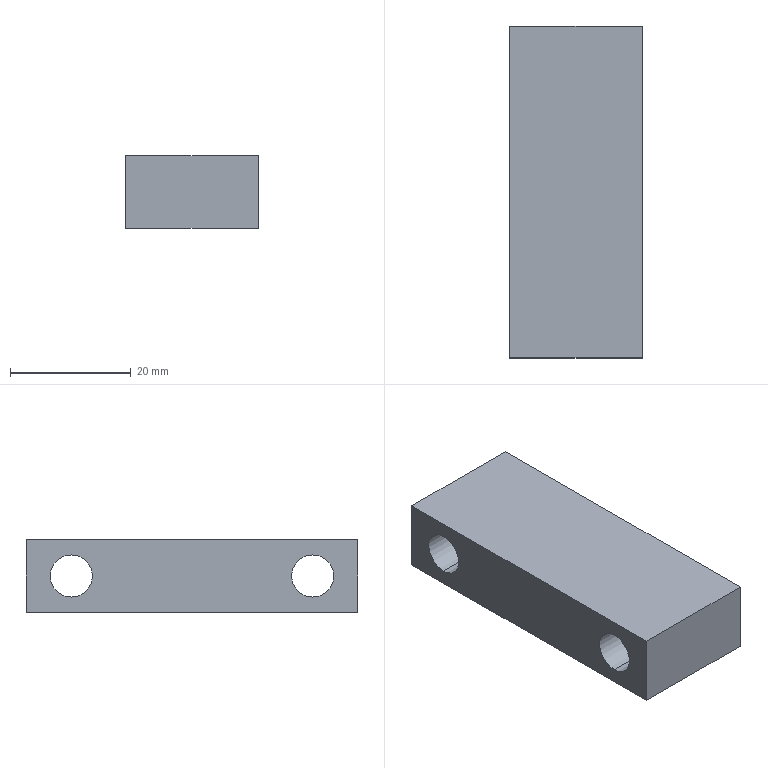Part | STEP file | CA-10-021Light Curtain Support Plate_Default | 1 solid | 10 faces | box 22 x 55 x 12 mm | volume 12827 mm3 | plane 6 | cylinder 4 | commonest cylinder face diameters 7 x4
STEP:
#1=CARTESIAN_POINT('',(0.,0.,0.));
#2=DIRECTION('',(0.,0.,1.));
#3=DIRECTION('',(1.,0.,0.));
#4=AXIS2_PLACEMENT_3D('',#1,#2,#3);
#5=CARTESIAN_POINT('',(11.,20.,9.5));
#6=VERTEX_POINT('',#5);
#7=CARTESIAN_POINT('',(-11.,20.,9.5));
#8=VERTEX_POINT('',#7);
#9=CARTESIAN_POINT('',(-11.,20.,9.5));
#10=DIRECTION('',(-1.,0.,0.));
#11=VECTOR('',#10,1.);
#12=LINE('',#9,#11);
#13=CARTESIAN_POINT('',(-11.,20.,6.));
#14=DIRECTION('',(-1.,0.,0.));
#15=DIRECTION('',(0.,0.,1.));
#16=AXIS2_PLACEMENT_3D('',#13,#14,#15);
#17=CYLINDRICAL_SURFACE('',#16,3.5);
#18=CARTESIAN_POINT('',(6.283,0.));
#19=DIRECTION('',(0.,1.));
#20=VECTOR('',#19,1.);
#21=LINE('',#18,#20);
#22=(GEOMETRIC_REPRESENTATION_CONTEXT(2)PARAMETRIC_REPRESENTATION_CONTEXT()REPRESENTATION_CONTEXT('',''));
#23=DEFINITIONAL_REPRESENTATION('',(#21),#22);
#24=PCURVE('',#17,#23);
#25=CARTESIAN_POINT('',(-11.,20.,6.));
#26=DIRECTION('',(-1.,0.,0.));
#27=DIRECTION('',(0.,0.,1.));
#28=AXIS2_PLACEMENT_3D('',#25,#26,#27);
#29=CYLINDRICAL_SURFACE('',#28,3.5);
#30=CARTESIAN_POINT('',(0.,0.));
#31=DIRECTION('',(0.,1.));
#32=VECTOR('',#31,1.);
#33=LINE('',#30,#32);
#34=(GEOMETRIC_REPRESENTATION_CONTEXT(2)PARAMETRIC_REPRESENTATION_CONTEXT()REPRESENTATION_CONTEXT('',''));
#35=DEFINITIONAL_REPRESENTATION('',(#33),#34);
#36=PCURVE('',#29,#35);
#37=SURFACE_CURVE('',#12,(#24,#36),.PCURVE_S1.);
#38=EDGE_CURVE('',#6,#8,#37,.T.);
#39=ORIENTED_EDGE('',*,*,#38,.T.);
#40=CARTESIAN_POINT('',(-11.,20.,2.5));
#41=VERTEX_POINT('',#40);
#42=CARTESIAN_POINT('',(-11.,20.,6.));
#43=DIRECTION('',(-1.,0.,0.));
#44=DIRECTION('',(0.,0.,1.));
#45=AXIS2_PLACEMENT_3D('',#42,#43,#44);
#46=CIRCLE('',#45,3.5);
#47=CARTESIAN_POINT('',(0.,0.));
#48=DIRECTION('',(1.,0.));
#49=VECTOR('',#48,1.);
#50=LINE('',#47,#49);
#51=(GEOMETRIC_REPRESENTATION_CONTEXT(2)PARAMETRIC_REPRESENTATION_CONTEXT()REPRESENTATION_CONTEXT('',''));
#52=DEFINITIONAL_REPRESENTATION('',(#50),#51);
#53=PCURVE('',#17,#52);
#54=CARTESIAN_POINT('',(-11.,27.5,12.));
#55=DIRECTION('',(1.,0.,0.));
#56=DIRECTION('',(0.,1.,0.));
#57=AXIS2_PLACEMENT_3D('',#54,#55,#56);
#58=PLANE('',#57);
#59=CARTESIAN_POINT('',(-7.5,-2.5));
#60=CARTESIAN_POINT('',(-1.438,-2.5));
#61=CARTESIAN_POINT('',(-4.469,-7.75));
#62=CARTESIAN_POINT('',(-7.5,-13.));
#63=CARTESIAN_POINT('',(-10.531,-7.75));
#64=CARTESIAN_POINT('',(-13.562,-2.5));
#65=CARTESIAN_POINT('',(-7.5,-2.5));
#66=(BOUNDED_CURVE()B_SPLINE_CURVE(2,(#59,#60,#61,#62,#63,#64,#65),.UNSPECIFIED.,.T.,.F.)B_SPLINE_CURVE_WITH_KNOTS((1,2,2,2,2,1),(-2.094,0.,2.094,4.189,6.283,8.378),.UNSPECIFIED.)CURVE()GEOMETRIC_REPRESENTATION_ITEM()RATIONAL_B_SPLINE_CURVE((1.,0.5,1.,0.5,1.,0.5,1.))REPRESENTATION_ITEM(''));
#67=(GEOMETRIC_REPRESENTATION_CONTEXT(2)PARAMETRIC_REPRESENTATION_CONTEXT()REPRESENTATION_CONTEXT('',''));
#68=DEFINITIONAL_REPRESENTATION('',(#66),#67);
#69=PCURVE('',#58,#68);
#70=SURFACE_CURVE('',#46,(#53,#69),.PCURVE_S1.);
#71=EDGE_CURVE('',#41,#8,#70,.T.);
#72=ORIENTED_EDGE('',*,*,#71,.F.);
#73=CARTESIAN_POINT('',(11.,20.,2.5));
#74=VERTEX_POINT('',#73);
#75=CARTESIAN_POINT('',(-11.,20.,2.5));
#76=DIRECTION('',(-1.,0.,0.));
#77=VECTOR('',#76,1.);
#78=LINE('',#75,#77);
#79=CARTESIAN_POINT('',(3.142,0.));
#80=DIRECTION('',(0.,1.));
#81=VECTOR('',#80,1.);
#82=LINE('',#79,#81);
#83=(GEOMETRIC_REPRESENTATION_CONTEXT(2)PARAMETRIC_REPRESENTATION_CONTEXT()REPRESENTATION_CONTEXT('',''));
#84=DEFINITIONAL_REPRESENTATION('',(#82),#83);
#85=PCURVE('',#17,#84);
#86=CARTESIAN_POINT('',(3.142,0.));
#87=DIRECTION('',(0.,1.));
#88=VECTOR('',#87,1.);
#89=LINE('',#86,#88);
#90=(GEOMETRIC_REPRESENTATION_CONTEXT(2)PARAMETRIC_REPRESENTATION_CONTEXT()REPRESENTATION_CONTEXT('',''));
#91=DEFINITIONAL_REPRESENTATION('',(#89),#90);
#92=PCURVE('',#29,#91);
#93=SURFACE_CURVE('',#78,(#85,#92),.PCURVE_S1.);
#94=EDGE_CURVE('',#74,#41,#93,.T.);
#95=ORIENTED_EDGE('',*,*,#94,.F.);
#96=CARTESIAN_POINT('',(11.,20.,6.));
#97=DIRECTION('',(-1.,0.,0.));
#98=DIRECTION('',(0.,0.,1.));
#99=AXIS2_PLACEMENT_3D('',#96,#97,#98);
#100=CIRCLE('',#99,3.5);
#101=CARTESIAN_POINT('',(0.,-22.));
#102=DIRECTION('',(1.,0.));
#103=VECTOR('',#102,1.);
#104=LINE('',#101,#103);
#105=(GEOMETRIC_REPRESENTATION_CONTEXT(2)PARAMETRIC_REPRESENTATION_CONTEXT()REPRESENTATION_CONTEXT('',''));
#106=DEFINITIONAL_REPRESENTATION('',(#104),#105);
#107=PCURVE('',#17,#106);
#108=CARTESIAN_POINT('',(11.,27.5,12.));
#109=DIRECTION('',(-1.,0.,0.));
#110=DIRECTION('',(0.,-1.,0.));
#111=AXIS2_PLACEMENT_3D('',#108,#109,#110);
#112=PLANE('',#111);
#113=CARTESIAN_POINT('',(7.5,-6.));
#114=DIRECTION('',(0.,1.));
#115=AXIS2_PLACEMENT_2D('',#113,#114);
#116=CIRCLE('',#115,3.5);
#117=(GEOMETRIC_REPRESENTATION_CONTEXT(2)PARAMETRIC_REPRESENTATION_CONTEXT()REPRESENTATION_CONTEXT('',''));
#118=DEFINITIONAL_REPRESENTATION('',(#116),#117);
#119=PCURVE('',#112,#118);
#120=SURFACE_CURVE('',#100,(#107,#119),.PCURVE_S1.);
#121=EDGE_CURVE('',#74,#6,#120,.T.);
#122=ORIENTED_EDGE('',*,*,#121,.T.);
#123=EDGE_LOOP('',(#39,#72,#95,#122));
#124=FACE_BOUND('',#123,.F.);
#125=ADVANCED_FACE('',(#124),#17,.F.);
#126=CARTESIAN_POINT('',(11.,-20.,9.5));
#127=VERTEX_POINT('',#126);
#128=CARTESIAN_POINT('',(-11.,-20.,9.5));
#129=VERTEX_POINT('',#128);
#130=CARTESIAN_POINT('',(-11.,-20.,9.5));
#131=DIRECTION('',(-1.,0.,0.));
#132=VECTOR('',#131,1.);
#133=LINE('',#130,#132);
#134=CARTESIAN_POINT('',(-11.,-20.,6.));
#135=DIRECTION('',(-1.,0.,0.));
#136=DIRECTION('',(0.,0.,1.));
#137=AXIS2_PLACEMENT_3D('',#134,#135,#136);
#138=CYLINDRICAL_SURFACE('',#137,3.5);
#139=CARTESIAN_POINT('',(6.283,0.));
#140=DIRECTION('',(0.,1.));
#141=VECTOR('',#140,1.);
#142=LINE('',#139,#141);
#143=(GEOMETRIC_REPRESENTATION_CONTEXT(2)PARAMETRIC_REPRESENTATION_CONTEXT()REPRESENTATION_CONTEXT('',''));
#144=DEFINITIONAL_REPRESENTATION('',(#142),#143);
#145=PCURVE('',#138,#144);
#146=CARTESIAN_POINT('',(-11.,-20.,6.));
#147=DIRECTION('',(-1.,0.,0.));
#148=DIRECTION('',(0.,0.,1.));
#149=AXIS2_PLACEMENT_3D('',#146,#147,#148);
#150=CYLINDRICAL_SURFACE('',#149,3.5);
#151=CARTESIAN_POINT('',(0.,0.));
#152=DIRECTION('',(0.,1.));
#153=VECTOR('',#152,1.);
#154=LINE('',#151,#153);
#155=(GEOMETRIC_REPRESENTATION_CONTEXT(2)PARAMETRIC_REPRESENTATION_CONTEXT()REPRESENTATION_CONTEXT('',''));
#156=DEFINITIONAL_REPRESENTATION('',(#154),#155);
#157=PCURVE('',#150,#156);
#158=SURFACE_CURVE('',#133,(#145,#157),.PCURVE_S1.);
#159=EDGE_CURVE('',#127,#129,#158,.T.);
#160=ORIENTED_EDGE('',*,*,#159,.T.);
#161=CARTESIAN_POINT('',(-11.,-20.,2.5));
#162=VERTEX_POINT('',#161);
#163=CARTESIAN_POINT('',(-11.,-20.,6.));
#164=DIRECTION('',(-1.,0.,0.));
#165=DIRECTION('',(0.,0.,1.));
#166=AXIS2_PLACEMENT_3D('',#163,#164,#165);
#167=CIRCLE('',#166,3.5);
#168=CARTESIAN_POINT('',(0.,0.));
#169=DIRECTION('',(1.,0.));
#170=VECTOR('',#169,1.);
#171=LINE('',#168,#170);
#172=(GEOMETRIC_REPRESENTATION_CONTEXT(2)PARAMETRIC_REPRESENTATION_CONTEXT()REPRESENTATION_CONTEXT('',''));
#173=DEFINITIONAL_REPRESENTATION('',(#171),#172);
#174=PCURVE('',#138,#173);
#175=CARTESIAN_POINT('',(-47.5,-2.5));
#176=CARTESIAN_POINT('',(-41.438,-2.5));
#177=CARTESIAN_POINT('',(-44.469,-7.75));
#178=CARTESIAN_POINT('',(-47.5,-13.));
#179=CARTESIAN_POINT('',(-50.531,-7.75));
#180=CARTESIAN_POINT('',(-53.562,-2.5));
#181=CARTESIAN_POINT('',(-47.5,-2.5));
#182=(BOUNDED_CURVE()B_SPLINE_CURVE(2,(#175,#176,#177,#178,#179,#180,#181),.UNSPECIFIED.,.T.,.F.)B_SPLINE_CURVE_WITH_KNOTS((1,2,2,2,2,1),(-2.094,0.,2.094,4.189,6.283,8.378),.UNSPECIFIED.)CURVE()GEOMETRIC_REPRESENTATION_ITEM()RATIONAL_B_SPLINE_CURVE((1.,0.5,1.,0.5,1.,0.5,1.))REPRESENTATION_ITEM(''));
#183=(GEOMETRIC_REPRESENTATION_CONTEXT(2)PARAMETRIC_REPRESENTATION_CONTEXT()REPRESENTATION_CONTEXT('',''));
#184=DEFINITIONAL_REPRESENTATION('',(#182),#183);
#185=PCURVE('',#58,#184);
#186=SURFACE_CURVE('',#167,(#174,#185),.PCURVE_S1.);
#187=EDGE_CURVE('',#162,#129,#186,.T.);
#188=ORIENTED_EDGE('',*,*,#187,.F.);
#189=CARTESIAN_POINT('',(11.,-20.,2.5));
#190=VERTEX_POINT('',#189);
#191=CARTESIAN_POINT('',(-11.,-20.,2.5));
#192=DIRECTION('',(-1.,0.,0.));
#193=VECTOR('',#192,1.);
#194=LINE('',#191,#193);
#195=CARTESIAN_POINT('',(3.142,0.));
#196=DIRECTION('',(0.,1.));
#197=VECTOR('',#196,1.);
#198=LINE('',#195,#197);
#199=(GEOMETRIC_REPRESENTATION_CONTEXT(2)PARAMETRIC_REPRESENTATION_CONTEXT()REPRESENTATION_CONTEXT('',''));
#200=DEFINITIONAL_REPRESENTATION('',(#198),#199);
#201=PCURVE('',#138,#200);
#202=CARTESIAN_POINT('',(3.142,0.));
#203=DIRECTION('',(0.,1.));
#204=VECTOR('',#203,1.);
#205=LINE('',#202,#204);
#206=(GEOMETRIC_REPRESENTATION_CONTEXT(2)PARAMETRIC_REPRESENTATION_CONTEXT()REPRESENTATION_CONTEXT('',''));
#207=DEFINITIONAL_REPRESENTATION('',(#205),#206);
#208=PCURVE('',#150,#207);
#209=SURFACE_CURVE('',#194,(#201,#208),.PCURVE_S1.);
#210=EDGE_CURVE('',#190,#162,#209,.T.);
#211=ORIENTED_EDGE('',*,*,#210,.F.);
#212=CARTESIAN_POINT('',(11.,-20.,6.));
#213=DIRECTION('',(-1.,0.,0.));
#214=DIRECTION('',(0.,0.,1.));
#215=AXIS2_PLACEMENT_3D('',#212,#213,#214);
#216=CIRCLE('',#215,3.5);
#217=CARTESIAN_POINT('',(0.,-22.));
#218=DIRECTION('',(1.,0.));
#219=VECTOR('',#218,1.);
#220=LINE('',#217,#219);
#221=(GEOMETRIC_REPRESENTATION_CONTEXT(2)PARAMETRIC_REPRESENTATION_CONTEXT()REPRESENTATION_CONTEXT('',''));
#222=DEFINITIONAL_REPRESENTATION('',(#220),#221);
#223=PCURVE('',#138,#222);
#224=CARTESIAN_POINT('',(47.5,-6.));
#225=DIRECTION('',(0.,1.));
#226=AXIS2_PLACEMENT_2D('',#224,#225);
#227=CIRCLE('',#226,3.5);
#228=(GEOMETRIC_REPRESENTATION_CONTEXT(2)PARAMETRIC_REPRESENTATION_CONTEXT()REPRESENTATION_CONTEXT('',''));
#229=DEFINITIONAL_REPRESENTATION('',(#227),#228);
#230=PCURVE('',#112,#229);
#231=SURFACE_CURVE('',#216,(#223,#230),.PCURVE_S1.);
#232=EDGE_CURVE('',#190,#127,#231,.T.);
#233=ORIENTED_EDGE('',*,*,#232,.T.);
#234=EDGE_LOOP('',(#160,#188,#211,#233));
#235=FACE_BOUND('',#234,.F.);
#236=ADVANCED_FACE('',(#235),#138,.F.);
#237=CARTESIAN_POINT('',(11.,20.,6.));
#238=DIRECTION('',(-1.,0.,0.));
#239=DIRECTION('',(0.,0.,1.));
#240=AXIS2_PLACEMENT_3D('',#237,#238,#239);
#241=CIRCLE('',#240,3.5);
#242=CARTESIAN_POINT('',(7.5,-6.));
#243=DIRECTION('',(0.,1.));
#244=AXIS2_PLACEMENT_2D('',#242,#243);
#245=CIRCLE('',#244,3.5);
#246=(GEOMETRIC_REPRESENTATION_CONTEXT(2)PARAMETRIC_REPRESENTATION_CONTEXT()REPRESENTATION_CONTEXT('',''));
#247=DEFINITIONAL_REPRESENTATION('',(#245),#246);
#248=PCURVE('',#112,#247);
#249=CARTESIAN_POINT('',(0.,-22.));
#250=DIRECTION('',(1.,0.));
#251=VECTOR('',#250,1.);
#252=LINE('',#249,#251);
#253=(GEOMETRIC_REPRESENTATION_CONTEXT(2)PARAMETRIC_REPRESENTATION_CONTEXT()REPRESENTATION_CONTEXT('',''));
#254=DEFINITIONAL_REPRESENTATION('',(#252),#253);
#255=PCURVE('',#29,#254);
#256=SURFACE_CURVE('',#241,(#248,#255),.PCURVE_S1.);
#257=EDGE_CURVE('',#6,#74,#256,.T.);
#258=ORIENTED_EDGE('',*,*,#257,.T.);
#259=ORIENTED_EDGE('',*,*,#121,.T.);
#260=EDGE_LOOP('',(#258,#259));
#261=FACE_BOUND('',#260,.T.);
#262=CARTESIAN_POINT('',(11.,-20.,6.));
#263=DIRECTION('',(-1.,0.,0.));
#264=DIRECTION('',(0.,0.,1.));
#265=AXIS2_PLACEMENT_3D('',#262,#263,#264);
#266=CIRCLE('',#265,3.5);
#267=CARTESIAN_POINT('',(47.5,-6.));
#268=DIRECTION('',(0.,1.));
#269=AXIS2_PLACEMENT_2D('',#267,#268);
#270=CIRCLE('',#269,3.5);
#271=(GEOMETRIC_REPRESENTATION_CONTEXT(2)PARAMETRIC_REPRESENTATION_CONTEXT()REPRESENTATION_CONTEXT('',''));
#272=DEFINITIONAL_REPRESENTATION('',(#270),#271);
#273=PCURVE('',#112,#272);
#274=CARTESIAN_POINT('',(0.,-22.));
#275=DIRECTION('',(1.,0.));
#276=VECTOR('',#275,1.);
#277=LINE('',#274,#276);
#278=(GEOMETRIC_REPRESENTATION_CONTEXT(2)PARAMETRIC_REPRESENTATION_CONTEXT()REPRESENTATION_CONTEXT('',''));
#279=DEFINITIONAL_REPRESENTATION('',(#277),#278);
#280=PCURVE('',#150,#279);
#281=SURFACE_CURVE('',#266,(#273,#280),.PCURVE_S1.);
#282=EDGE_CURVE('',#127,#190,#281,.T.);
#283=ORIENTED_EDGE('',*,*,#282,.T.);
#284=ORIENTED_EDGE('',*,*,#232,.T.);
#285=EDGE_LOOP('',(#283,#284));
#286=FACE_BOUND('',#285,.T.);
#287=CARTESIAN_POINT('',(11.,-27.5,0.));
#288=VERTEX_POINT('',#287);
#289=CARTESIAN_POINT('',(11.,27.5,0.));
#290=VERTEX_POINT('',#289);
#291=CARTESIAN_POINT('',(11.,27.5,0.));
#292=DIRECTION('',(0.,1.,0.));
#293=VECTOR('',#292,1.);
#294=LINE('',#291,#293);
#295=CARTESIAN_POINT('',(0.,-12.));
#296=DIRECTION('',(-1.,0.));
#297=VECTOR('',#296,1.);
#298=LINE('',#295,#297);
#299=(GEOMETRIC_REPRESENTATION_CONTEXT(2)PARAMETRIC_REPRESENTATION_CONTEXT()REPRESENTATION_CONTEXT('',''));
#300=DEFINITIONAL_REPRESENTATION('',(#298),#299);
#301=PCURVE('',#112,#300);
#302=CARTESIAN_POINT('',(0.,0.,0.));
#303=DIRECTION('',(0.,0.,1.));
#304=DIRECTION('',(1.,0.,0.));
#305=AXIS2_PLACEMENT_3D('',#302,#303,#304);
#306=PLANE('',#305);
#307=CARTESIAN_POINT('',(11.,27.5));
#308=DIRECTION('',(0.,1.));
#309=VECTOR('',#308,1.);
#310=LINE('',#307,#309);
#311=(GEOMETRIC_REPRESENTATION_CONTEXT(2)PARAMETRIC_REPRESENTATION_CONTEXT()REPRESENTATION_CONTEXT('',''));
#312=DEFINITIONAL_REPRESENTATION('',(#310),#311);
#313=PCURVE('',#306,#312);
#314=SURFACE_CURVE('',#294,(#301,#313),.PCURVE_S1.);
#315=EDGE_CURVE('',#288,#290,#314,.T.);
#316=ORIENTED_EDGE('',*,*,#315,.T.);
#317=CARTESIAN_POINT('',(11.,27.5,12.));
#318=VERTEX_POINT('',#317);
#319=CARTESIAN_POINT('',(11.,27.5,12.));
#320=DIRECTION('',(0.,0.,-1.));
#321=VECTOR('',#320,1.);
#322=LINE('',#319,#321);
#323=CARTESIAN_POINT('',(0.,0.));
#324=DIRECTION('',(0.,-1.));
#325=VECTOR('',#324,1.);
#326=LINE('',#323,#325);
#327=(GEOMETRIC_REPRESENTATION_CONTEXT(2)PARAMETRIC_REPRESENTATION_CONTEXT()REPRESENTATION_CONTEXT('',''));
#328=DEFINITIONAL_REPRESENTATION('',(#326),#327);
#329=PCURVE('',#112,#328);
#330=CARTESIAN_POINT('',(-11.,27.5,12.));
#331=DIRECTION('',(0.,-1.,0.));
#332=DIRECTION('',(0.,0.,-1.));
#333=AXIS2_PLACEMENT_3D('',#330,#331,#332);
#334=PLANE('',#333);
#335=CARTESIAN_POINT('',(0.,22.));
#336=DIRECTION('',(1.,0.));
#337=VECTOR('',#336,1.);
#338=LINE('',#335,#337);
#339=(GEOMETRIC_REPRESENTATION_CONTEXT(2)PARAMETRIC_REPRESENTATION_CONTEXT()REPRESENTATION_CONTEXT('',''));
#340=DEFINITIONAL_REPRESENTATION('',(#338),#339);
#341=PCURVE('',#334,#340);
#342=SURFACE_CURVE('',#322,(#329,#341),.PCURVE_S1.);
#343=EDGE_CURVE('',#318,#290,#342,.T.);
#344=ORIENTED_EDGE('',*,*,#343,.F.);
#345=CARTESIAN_POINT('',(11.,-27.5,12.));
#346=VERTEX_POINT('',#345);
#347=CARTESIAN_POINT('',(11.,27.5,12.));
#348=DIRECTION('',(0.,1.,0.));
#349=VECTOR('',#348,1.);
#350=LINE('',#347,#349);
#351=CARTESIAN_POINT('',(0.,0.));
#352=DIRECTION('',(-1.,0.));
#353=VECTOR('',#352,1.);
#354=LINE('',#351,#353);
#355=(GEOMETRIC_REPRESENTATION_CONTEXT(2)PARAMETRIC_REPRESENTATION_CONTEXT()REPRESENTATION_CONTEXT('',''));
#356=DEFINITIONAL_REPRESENTATION('',(#354),#355);
#357=PCURVE('',#112,#356);
#358=CARTESIAN_POINT('',(0.,0.,12.));
#359=DIRECTION('',(0.,0.,1.));
#360=DIRECTION('',(1.,0.,0.));
#361=AXIS2_PLACEMENT_3D('',#358,#359,#360);
#362=PLANE('',#361);
#363=CARTESIAN_POINT('',(11.,27.5));
#364=DIRECTION('',(0.,1.));
#365=VECTOR('',#364,1.);
#366=LINE('',#363,#365);
#367=(GEOMETRIC_REPRESENTATION_CONTEXT(2)PARAMETRIC_REPRESENTATION_CONTEXT()REPRESENTATION_CONTEXT('',''));
#368=DEFINITIONAL_REPRESENTATION('',(#366),#367);
#369=PCURVE('',#362,#368);
#370=SURFACE_CURVE('',#350,(#357,#369),.PCURVE_S1.);
#371=EDGE_CURVE('',#346,#318,#370,.T.);
#372=ORIENTED_EDGE('',*,*,#371,.F.);
#373=CARTESIAN_POINT('',(11.,-27.5,12.));
#374=DIRECTION('',(0.,0.,-1.));
#375=VECTOR('',#374,1.);
#376=LINE('',#373,#375);
#377=CARTESIAN_POINT('',(55.,0.));
#378=DIRECTION('',(0.,-1.));
#379=VECTOR('',#378,1.);
#380=LINE('',#377,#379);
#381=(GEOMETRIC_REPRESENTATION_CONTEXT(2)PARAMETRIC_REPRESENTATION_CONTEXT()REPRESENTATION_CONTEXT('',''));
#382=DEFINITIONAL_REPRESENTATION('',(#380),#381);
#383=PCURVE('',#112,#382);
#384=CARTESIAN_POINT('',(-11.,-27.5,12.));
#385=DIRECTION('',(0.,1.,0.));
#386=DIRECTION('',(0.,0.,1.));
#387=AXIS2_PLACEMENT_3D('',#384,#385,#386);
#388=PLANE('',#387);
#389=CARTESIAN_POINT('',(0.,22.));
#390=DIRECTION('',(-1.,0.));
#391=VECTOR('',#390,1.);
#392=LINE('',#389,#391);
#393=(GEOMETRIC_REPRESENTATION_CONTEXT(2)PARAMETRIC_REPRESENTATION_CONTEXT()REPRESENTATION_CONTEXT('',''));
#394=DEFINITIONAL_REPRESENTATION('',(#392),#393);
#395=PCURVE('',#388,#394);
#396=SURFACE_CURVE('',#376,(#383,#395),.PCURVE_S1.);
#397=EDGE_CURVE('',#346,#288,#396,.T.);
#398=ORIENTED_EDGE('',*,*,#397,.T.);
#399=EDGE_LOOP('',(#316,#344,#372,#398));
#400=FACE_BOUND('',#399,.T.);
#401=ADVANCED_FACE('',(#261,#286,#400),#112,.F.);
#402=CARTESIAN_POINT('',(-11.,27.5,0.));
#403=VERTEX_POINT('',#402);
#404=CARTESIAN_POINT('',(-11.,27.5,0.));
#405=DIRECTION('',(-1.,0.,0.));
#406=VECTOR('',#405,1.);
#407=LINE('',#404,#406);
#408=CARTESIAN_POINT('',(12.,0.));
#409=DIRECTION('',(0.,-1.));
#410=VECTOR('',#409,1.);
#411=LINE('',#408,#410);
#412=(GEOMETRIC_REPRESENTATION_CONTEXT(2)PARAMETRIC_REPRESENTATION_CONTEXT()REPRESENTATION_CONTEXT('',''));
#413=DEFINITIONAL_REPRESENTATION('',(#411),#412);
#414=PCURVE('',#334,#413);
#415=CARTESIAN_POINT('',(-11.,27.5));
#416=DIRECTION('',(-1.,0.));
#417=VECTOR('',#416,1.);
#418=LINE('',#415,#417);
#419=(GEOMETRIC_REPRESENTATION_CONTEXT(2)PARAMETRIC_REPRESENTATION_CONTEXT()REPRESENTATION_CONTEXT('',''));
#420=DEFINITIONAL_REPRESENTATION('',(#418),#419);
#421=PCURVE('',#306,#420);
#422=SURFACE_CURVE('',#407,(#414,#421),.PCURVE_S1.);
#423=EDGE_CURVE('',#290,#403,#422,.T.);
#424=ORIENTED_EDGE('',*,*,#423,.T.);
#425=CARTESIAN_POINT('',(-11.,27.5,12.));
#426=VERTEX_POINT('',#425);
#427=CARTESIAN_POINT('',(-11.,27.5,12.));
#428=DIRECTION('',(0.,0.,-1.));
#429=VECTOR('',#428,1.);
#430=LINE('',#427,#429);
#431=CARTESIAN_POINT('',(0.,0.));
#432=DIRECTION('',(1.,0.));
#433=VECTOR('',#432,1.);
#434=LINE('',#431,#433);
#435=(GEOMETRIC_REPRESENTATION_CONTEXT(2)PARAMETRIC_REPRESENTATION_CONTEXT()REPRESENTATION_CONTEXT('',''));
#436=DEFINITIONAL_REPRESENTATION('',(#434),#435);
#437=PCURVE('',#334,#436);
#438=CARTESIAN_POINT('',(0.,0.));
#439=DIRECTION('',(0.,-1.));
#440=VECTOR('',#439,1.);
#441=LINE('',#438,#440);
#442=(GEOMETRIC_REPRESENTATION_CONTEXT(2)PARAMETRIC_REPRESENTATION_CONTEXT()REPRESENTATION_CONTEXT('',''));
#443=DEFINITIONAL_REPRESENTATION('',(#441),#442);
#444=PCURVE('',#58,#443);
#445=SURFACE_CURVE('',#430,(#437,#444),.PCURVE_S1.);
#446=EDGE_CURVE('',#426,#403,#445,.T.);
#447=ORIENTED_EDGE('',*,*,#446,.F.);
#448=CARTESIAN_POINT('',(-11.,27.5,12.));
#449=DIRECTION('',(-1.,0.,0.));
#450=VECTOR('',#449,1.);
#451=LINE('',#448,#450);
#452=CARTESIAN_POINT('',(0.,0.));
#453=DIRECTION('',(0.,-1.));
#454=VECTOR('',#453,1.);
#455=LINE('',#452,#454);
#456=(GEOMETRIC_REPRESENTATION_CONTEXT(2)PARAMETRIC_REPRESENTATION_CONTEXT()REPRESENTATION_CONTEXT('',''));
#457=DEFINITIONAL_REPRESENTATION('',(#455),#456);
#458=PCURVE('',#334,#457);
#459=CARTESIAN_POINT('',(-11.,27.5));
#460=DIRECTION('',(-1.,0.));
#461=VECTOR('',#460,1.);
#462=LINE('',#459,#461);
#463=(GEOMETRIC_REPRESENTATION_CONTEXT(2)PARAMETRIC_REPRESENTATION_CONTEXT()REPRESENTATION_CONTEXT('',''));
#464=DEFINITIONAL_REPRESENTATION('',(#462),#463);
#465=PCURVE('',#362,#464);
#466=SURFACE_CURVE('',#451,(#458,#465),.PCURVE_S1.);
#467=EDGE_CURVE('',#318,#426,#466,.T.);
#468=ORIENTED_EDGE('',*,*,#467,.F.);
#469=ORIENTED_EDGE('',*,*,#343,.T.);
#470=EDGE_LOOP('',(#424,#447,#468,#469));
#471=FACE_BOUND('',#470,.T.);
#472=ADVANCED_FACE('',(#471),#334,.F.);
#473=CARTESIAN_POINT('',(-11.,20.,6.));
#474=DIRECTION('',(-1.,0.,0.));
#475=DIRECTION('',(0.,0.,1.));
#476=AXIS2_PLACEMENT_3D('',#473,#474,#475);
#477=CIRCLE('',#476,3.5);
#478=CARTESIAN_POINT('',(-7.5,-2.5));
#479=CARTESIAN_POINT('',(-1.438,-2.5));
#480=CARTESIAN_POINT('',(-4.469,-7.75));
#481=CARTESIAN_POINT('',(-7.5,-13.));
#482=CARTESIAN_POINT('',(-10.531,-7.75));
#483=CARTESIAN_POINT('',(-13.562,-2.5));
#484=CARTESIAN_POINT('',(-7.5,-2.5));
#485=(BOUNDED_CURVE()B_SPLINE_CURVE(2,(#478,#479,#480,#481,#482,#483,#484),.UNSPECIFIED.,.T.,.F.)B_SPLINE_CURVE_WITH_KNOTS((1,2,2,2,2,1),(-2.094,0.,2.094,4.189,6.283,8.378),.UNSPECIFIED.)CURVE()GEOMETRIC_REPRESENTATION_ITEM()RATIONAL_B_SPLINE_CURVE((1.,0.5,1.,0.5,1.,0.5,1.))REPRESENTATION_ITEM(''));
#486=(GEOMETRIC_REPRESENTATION_CONTEXT(2)PARAMETRIC_REPRESENTATION_CONTEXT()REPRESENTATION_CONTEXT('',''));
#487=DEFINITIONAL_REPRESENTATION('',(#485),#486);
#488=PCURVE('',#58,#487);
#489=CARTESIAN_POINT('',(0.,0.));
#490=DIRECTION('',(1.,0.));
#491=VECTOR('',#490,1.);
#492=LINE('',#489,#491);
#493=(GEOMETRIC_REPRESENTATION_CONTEXT(2)PARAMETRIC_REPRESENTATION_CONTEXT()REPRESENTATION_CONTEXT('',''));
#494=DEFINITIONAL_REPRESENTATION('',(#492),#493);
#495=PCURVE('',#29,#494);
#496=SURFACE_CURVE('',#477,(#488,#495),.PCURVE_S1.);
#497=EDGE_CURVE('',#8,#41,#496,.T.);
#498=ORIENTED_EDGE('',*,*,#497,.F.);
#499=ORIENTED_EDGE('',*,*,#71,.F.);
#500=EDGE_LOOP('',(#498,#499));
#501=FACE_BOUND('',#500,.T.);
#502=CARTESIAN_POINT('',(-11.,-20.,6.));
#503=DIRECTION('',(-1.,0.,0.));
#504=DIRECTION('',(0.,0.,1.));
#505=AXIS2_PLACEMENT_3D('',#502,#503,#504);
#506=CIRCLE('',#505,3.5);
#507=CARTESIAN_POINT('',(-47.5,-2.5));
#508=CARTESIAN_POINT('',(-41.438,-2.5));
#509=CARTESIAN_POINT('',(-44.469,-7.75));
#510=CARTESIAN_POINT('',(-47.5,-13.));
#511=CARTESIAN_POINT('',(-50.531,-7.75));
#512=CARTESIAN_POINT('',(-53.562,-2.5));
#513=CARTESIAN_POINT('',(-47.5,-2.5));
#514=(BOUNDED_CURVE()B_SPLINE_CURVE(2,(#507,#508,#509,#510,#511,#512,#513),.UNSPECIFIED.,.T.,.F.)B_SPLINE_CURVE_WITH_KNOTS((1,2,2,2,2,1),(-2.094,0.,2.094,4.189,6.283,8.378),.UNSPECIFIED.)CURVE()GEOMETRIC_REPRESENTATION_ITEM()RATIONAL_B_SPLINE_CURVE((1.,0.5,1.,0.5,1.,0.5,1.))REPRESENTATION_ITEM(''));
#515=(GEOMETRIC_REPRESENTATION_CONTEXT(2)PARAMETRIC_REPRESENTATION_CONTEXT()REPRESENTATION_CONTEXT('',''));
#516=DEFINITIONAL_REPRESENTATION('',(#514),#515);
#517=PCURVE('',#58,#516);
#518=CARTESIAN_POINT('',(0.,0.));
#519=DIRECTION('',(1.,0.));
#520=VECTOR('',#519,1.);
#521=LINE('',#518,#520);
#522=(GEOMETRIC_REPRESENTATION_CONTEXT(2)PARAMETRIC_REPRESENTATION_CONTEXT()REPRESENTATION_CONTEXT('',''));
#523=DEFINITIONAL_REPRESENTATION('',(#521),#522);
#524=PCURVE('',#150,#523);
#525=SURFACE_CURVE('',#506,(#517,#524),.PCURVE_S1.);
#526=EDGE_CURVE('',#129,#162,#525,.T.);
#527=ORIENTED_EDGE('',*,*,#526,.F.);
#528=ORIENTED_EDGE('',*,*,#187,.F.);
#529=EDGE_LOOP('',(#527,#528));
#530=FACE_BOUND('',#529,.T.);
#531=CARTESIAN_POINT('',(-11.,-27.5,0.));
#532=VERTEX_POINT('',#531);
#533=CARTESIAN_POINT('',(-11.,27.5,0.));
#534=DIRECTION('',(0.,-1.,0.));
#535=VECTOR('',#534,1.);
#536=LINE('',#533,#535);
#537=CARTESIAN_POINT('',(0.,-12.));
#538=DIRECTION('',(-1.,0.));
#539=VECTOR('',#538,1.);
#540=LINE('',#537,#539);
#541=(GEOMETRIC_REPRESENTATION_CONTEXT(2)PARAMETRIC_REPRESENTATION_CONTEXT()REPRESENTATION_CONTEXT('',''));
#542=DEFINITIONAL_REPRESENTATION('',(#540),#541);
#543=PCURVE('',#58,#542);
#544=CARTESIAN_POINT('',(-11.,27.5));
#545=DIRECTION('',(0.,-1.));
#546=VECTOR('',#545,1.);
#547=LINE('',#544,#546);
#548=(GEOMETRIC_REPRESENTATION_CONTEXT(2)PARAMETRIC_REPRESENTATION_CONTEXT()REPRESENTATION_CONTEXT('',''));
#549=DEFINITIONAL_REPRESENTATION('',(#547),#548);
#550=PCURVE('',#306,#549);
#551=SURFACE_CURVE('',#536,(#543,#550),.PCURVE_S1.);
#552=EDGE_CURVE('',#403,#532,#551,.T.);
#553=ORIENTED_EDGE('',*,*,#552,.T.);
#554=CARTESIAN_POINT('',(-11.,-27.5,12.));
#555=VERTEX_POINT('',#554);
#556=CARTESIAN_POINT('',(-11.,-27.5,12.));
#557=DIRECTION('',(0.,0.,-1.));
#558=VECTOR('',#557,1.);
#559=LINE('',#556,#558);
#560=CARTESIAN_POINT('',(-55.,0.));
#561=DIRECTION('',(0.,-1.));
#562=VECTOR('',#561,1.);
#563=LINE('',#560,#562);
#564=(GEOMETRIC_REPRESENTATION_CONTEXT(2)PARAMETRIC_REPRESENTATION_CONTEXT()REPRESENTATION_CONTEXT('',''));
#565=DEFINITIONAL_REPRESENTATION('',(#563),#564);
#566=PCURVE('',#58,#565);
#567=CARTESIAN_POINT('',(0.,0.));
#568=DIRECTION('',(-1.,0.));
#569=VECTOR('',#568,1.);
#570=LINE('',#567,#569);
#571=(GEOMETRIC_REPRESENTATION_CONTEXT(2)PARAMETRIC_REPRESENTATION_CONTEXT()REPRESENTATION_CONTEXT('',''));
#572=DEFINITIONAL_REPRESENTATION('',(#570),#571);
#573=PCURVE('',#388,#572);
#574=SURFACE_CURVE('',#559,(#566,#573),.PCURVE_S1.);
#575=EDGE_CURVE('',#555,#532,#574,.T.);
#576=ORIENTED_EDGE('',*,*,#575,.F.);
#577=CARTESIAN_POINT('',(-11.,27.5,12.));
#578=DIRECTION('',(0.,-1.,0.));
#579=VECTOR('',#578,1.);
#580=LINE('',#577,#579);
#581=CARTESIAN_POINT('',(0.,0.));
#582=DIRECTION('',(-1.,0.));
#583=VECTOR('',#582,1.);
#584=LINE('',#581,#583);
#585=(GEOMETRIC_REPRESENTATION_CONTEXT(2)PARAMETRIC_REPRESENTATION_CONTEXT()REPRESENTATION_CONTEXT('',''));
#586=DEFINITIONAL_REPRESENTATION('',(#584),#585);
#587=PCURVE('',#58,#586);
#588=CARTESIAN_POINT('',(-11.,27.5));
#589=DIRECTION('',(0.,-1.));
#590=VECTOR('',#589,1.);
#591=LINE('',#588,#590);
#592=(GEOMETRIC_REPRESENTATION_CONTEXT(2)PARAMETRIC_REPRESENTATION_CONTEXT()REPRESENTATION_CONTEXT('',''));
#593=DEFINITIONAL_REPRESENTATION('',(#591),#592);
#594=PCURVE('',#362,#593);
#595=SURFACE_CURVE('',#580,(#587,#594),.PCURVE_S1.);
#596=EDGE_CURVE('',#426,#555,#595,.T.);
#597=ORIENTED_EDGE('',*,*,#596,.F.);
#598=ORIENTED_EDGE('',*,*,#446,.T.);
#599=EDGE_LOOP('',(#553,#576,#597,#598));
#600=FACE_BOUND('',#599,.T.);
#601=ADVANCED_FACE('',(#501,#530,#600),#58,.F.);
#602=CARTESIAN_POINT('',(-11.,-27.5,0.));
#603=DIRECTION('',(1.,0.,0.));
#604=VECTOR('',#603,1.);
#605=LINE('',#602,#604);
#606=CARTESIAN_POINT('',(-12.,0.));
#607=DIRECTION('',(0.,1.));
#608=VECTOR('',#607,1.);
#609=LINE('',#606,#608);
#610=(GEOMETRIC_REPRESENTATION_CONTEXT(2)PARAMETRIC_REPRESENTATION_CONTEXT()REPRESENTATION_CONTEXT('',''));
#611=DEFINITIONAL_REPRESENTATION('',(#609),#610);
#612=PCURVE('',#388,#611);
#613=CARTESIAN_POINT('',(-11.,-27.5));
#614=DIRECTION('',(1.,0.));
#615=VECTOR('',#614,1.);
#616=LINE('',#613,#615);
#617=(GEOMETRIC_REPRESENTATION_CONTEXT(2)PARAMETRIC_REPRESENTATION_CONTEXT()REPRESENTATION_CONTEXT('',''));
#618=DEFINITIONAL_REPRESENTATION('',(#616),#617);
#619=PCURVE('',#306,#618);
#620=SURFACE_CURVE('',#605,(#612,#619),.PCURVE_S1.);
#621=EDGE_CURVE('',#532,#288,#620,.T.);
#622=ORIENTED_EDGE('',*,*,#621,.T.);
#623=ORIENTED_EDGE('',*,*,#397,.F.);
#624=CARTESIAN_POINT('',(-11.,-27.5,12.));
#625=DIRECTION('',(1.,0.,0.));
#626=VECTOR('',#625,1.);
#627=LINE('',#624,#626);
#628=CARTESIAN_POINT('',(0.,0.));
#629=DIRECTION('',(0.,1.));
#630=VECTOR('',#629,1.);
#631=LINE('',#628,#630);
#632=(GEOMETRIC_REPRESENTATION_CONTEXT(2)PARAMETRIC_REPRESENTATION_CONTEXT()REPRESENTATION_CONTEXT('',''));
#633=DEFINITIONAL_REPRESENTATION('',(#631),#632);
#634=PCURVE('',#388,#633);
#635=CARTESIAN_POINT('',(-11.,-27.5));
#636=DIRECTION('',(1.,0.));
#637=VECTOR('',#636,1.);
#638=LINE('',#635,#637);
#639=(GEOMETRIC_REPRESENTATION_CONTEXT(2)PARAMETRIC_REPRESENTATION_CONTEXT()REPRESENTATION_CONTEXT('',''));
#640=DEFINITIONAL_REPRESENTATION('',(#638),#639);
#641=PCURVE('',#362,#640);
#642=SURFACE_CURVE('',#627,(#634,#641),.PCURVE_S1.);
#643=EDGE_CURVE('',#555,#346,#642,.T.);
#644=ORIENTED_EDGE('',*,*,#643,.F.);
#645=ORIENTED_EDGE('',*,*,#575,.T.);
#646=EDGE_LOOP('',(#622,#623,#644,#645));
#647=FACE_BOUND('',#646,.T.);
#648=ADVANCED_FACE('',(#647),#388,.F.);
#649=ORIENTED_EDGE('',*,*,#371,.T.);
#650=ORIENTED_EDGE('',*,*,#467,.T.);
#651=ORIENTED_EDGE('',*,*,#596,.T.);
#652=ORIENTED_EDGE('',*,*,#643,.T.);
#653=EDGE_LOOP('',(#649,#650,#651,#652));
#654=FACE_BOUND('',#653,.T.);
#655=ADVANCED_FACE('',(#654),#362,.T.);
#656=ORIENTED_EDGE('',*,*,#315,.F.);
#657=ORIENTED_EDGE('',*,*,#621,.F.);
#658=ORIENTED_EDGE('',*,*,#552,.F.);
#659=ORIENTED_EDGE('',*,*,#423,.F.);
#660=EDGE_LOOP('',(#656,#657,#658,#659));
#661=FACE_BOUND('',#660,.T.);
#662=ADVANCED_FACE('',(#661),#306,.F.);
#663=ORIENTED_EDGE('',*,*,#526,.F.);
#664=ORIENTED_EDGE('',*,*,#159,.F.);
#665=ORIENTED_EDGE('',*,*,#282,.T.);
#666=ORIENTED_EDGE('',*,*,#210,.T.);
#667=EDGE_LOOP('',(#663,#664,#665,#666));
#668=FACE_BOUND('',#667,.F.);
#669=ADVANCED_FACE('',(#668),#150,.F.);
#670=ORIENTED_EDGE('',*,*,#497,.F.);
#671=ORIENTED_EDGE('',*,*,#38,.F.);
#672=ORIENTED_EDGE('',*,*,#257,.T.);
#673=ORIENTED_EDGE('',*,*,#94,.T.);
#674=EDGE_LOOP('',(#670,#671,#672,#673));
#675=FACE_BOUND('',#674,.F.);
#676=ADVANCED_FACE('',(#675),#29,.F.);
#677=CLOSED_SHELL('',(#125,#236,#401,#472,#601,#648,#655,#662,#669,#676));
#678=MANIFOLD_SOLID_BREP('',#677);
#679=(LENGTH_UNIT()NAMED_UNIT(*)SI_UNIT(.MILLI.,.METRE.));
#680=UNCERTAINTY_MEASURE_WITH_UNIT(LENGTH_MEASURE(0.0000001),#679,'','');
#681=(NAMED_UNIT(*)PLANE_ANGLE_UNIT()SI_UNIT($,.RADIAN.));
#682=(NAMED_UNIT(*)SI_UNIT($,.STERADIAN.)SOLID_ANGLE_UNIT());
#683=(GEOMETRIC_REPRESENTATION_CONTEXT(3)GLOBAL_UNCERTAINTY_ASSIGNED_CONTEXT((#680))GLOBAL_UNIT_ASSIGNED_CONTEXT((#679,#681,#682))REPRESENTATION_CONTEXT('',''));
#684=ADVANCED_BREP_SHAPE_REPRESENTATION('',(#4,#678),#683);